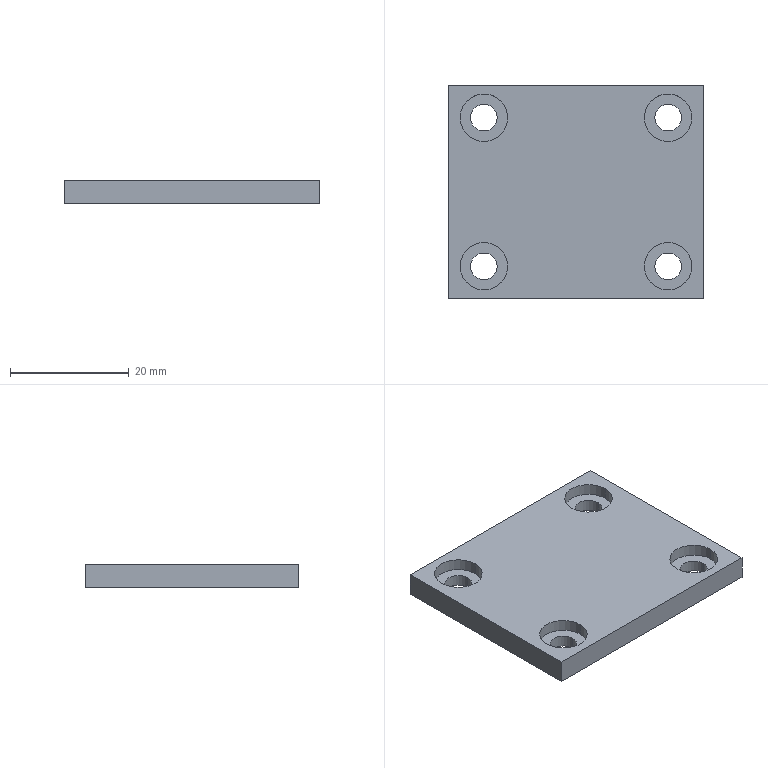Part | SolidWorks | features BaseBody 1 | 1 solid | 26 faces | box 43 x 36 x 4 mm | volume 5663 mm3 | cylinder 16 | plane 10 | commonest cylinder face diameters 4.5 x8 8 x8
STEP:
#1=CARTESIAN_POINT('',(-13.25,-12.5,0.));
#2=VERTEX_POINT('',#1);
#3=CARTESIAN_POINT('',(-17.75,-12.5,0.));
#4=VERTEX_POINT('',#3);
#5=CARTESIAN_POINT('',(-15.5,-12.5,0.));
#6=DIRECTION('',(0.,0.,-1.));
#7=DIRECTION('',(1.,0.,0.));
#8=AXIS2_PLACEMENT_3D('',#5,#6,#7);
#9=CIRCLE('',#8,2.25);
#10=EDGE_CURVE('',#2,#4,#9,.T.);
#11=ORIENTED_EDGE('',*,*,#10,.T.);
#12=CARTESIAN_POINT('',(-17.75,-12.5,2.));
#13=VERTEX_POINT('',#12);
#14=CARTESIAN_POINT('',(-17.75,-12.5,4.));
#15=DIRECTION('',(0.,0.,1.));
#16=VECTOR('',#15,1000.);
#17=LINE('',#14,#16);
#18=EDGE_CURVE('',#4,#13,#17,.T.);
#19=ORIENTED_EDGE('',*,*,#18,.T.);
#20=CARTESIAN_POINT('',(-13.25,-12.5,2.));
#21=VERTEX_POINT('',#20);
#22=CARTESIAN_POINT('',(-15.5,-12.5,2.));
#23=DIRECTION('',(0.,0.,-1.));
#24=DIRECTION('',(1.,0.,0.));
#25=AXIS2_PLACEMENT_3D('',#22,#23,#24);
#26=CIRCLE('',#25,2.25);
#27=EDGE_CURVE('',#21,#13,#26,.T.);
#28=ORIENTED_EDGE('',*,*,#27,.F.);
#29=CARTESIAN_POINT('',(-13.25,-12.5,4.));
#30=DIRECTION('',(0.,0.,1.));
#31=VECTOR('',#30,1000.);
#32=LINE('',#29,#31);
#33=EDGE_CURVE('',#2,#21,#32,.T.);
#34=ORIENTED_EDGE('',*,*,#33,.F.);
#35=EDGE_LOOP('',(#11,#19,#28,#34));
#36=FACE_OUTER_BOUND('',#35,.T.);
#37=CARTESIAN_POINT('',(-15.5,-12.5,4.));
#38=DIRECTION('',(0.,0.,1.));
#39=DIRECTION('',(1.,0.,0.));
#40=AXIS2_PLACEMENT_3D('',#37,#38,#39);
#41=CYLINDRICAL_SURFACE('',#40,2.25);
#42=ADVANCED_FACE('',(#36),#41,.F.);
#43=CARTESIAN_POINT('',(17.75,-12.5,0.));
#44=VERTEX_POINT('',#43);
#45=CARTESIAN_POINT('',(13.25,-12.5,0.));
#46=VERTEX_POINT('',#45);
#47=CARTESIAN_POINT('',(15.5,-12.5,0.));
#48=DIRECTION('',(0.,0.,-1.));
#49=DIRECTION('',(1.,0.,0.));
#50=AXIS2_PLACEMENT_3D('',#47,#48,#49);
#51=CIRCLE('',#50,2.25);
#52=EDGE_CURVE('',#44,#46,#51,.T.);
#53=ORIENTED_EDGE('',*,*,#52,.T.);
#54=CARTESIAN_POINT('',(13.25,-12.5,2.));
#55=VERTEX_POINT('',#54);
#56=CARTESIAN_POINT('',(13.25,-12.5,4.));
#57=DIRECTION('',(0.,0.,1.));
#58=VECTOR('',#57,1000.);
#59=LINE('',#56,#58);
#60=EDGE_CURVE('',#46,#55,#59,.T.);
#61=ORIENTED_EDGE('',*,*,#60,.T.);
#62=CARTESIAN_POINT('',(17.75,-12.5,2.));
#63=VERTEX_POINT('',#62);
#64=CARTESIAN_POINT('',(15.5,-12.5,2.));
#65=DIRECTION('',(0.,0.,-1.));
#66=DIRECTION('',(1.,0.,0.));
#67=AXIS2_PLACEMENT_3D('',#64,#65,#66);
#68=CIRCLE('',#67,2.25);
#69=EDGE_CURVE('',#63,#55,#68,.T.);
#70=ORIENTED_EDGE('',*,*,#69,.F.);
#71=CARTESIAN_POINT('',(17.75,-12.5,4.));
#72=DIRECTION('',(0.,0.,1.));
#73=VECTOR('',#72,1000.);
#74=LINE('',#71,#73);
#75=EDGE_CURVE('',#44,#63,#74,.T.);
#76=ORIENTED_EDGE('',*,*,#75,.F.);
#77=EDGE_LOOP('',(#53,#61,#70,#76));
#78=FACE_OUTER_BOUND('',#77,.T.);
#79=CARTESIAN_POINT('',(15.5,-12.5,4.));
#80=DIRECTION('',(0.,0.,1.));
#81=DIRECTION('',(1.,0.,0.));
#82=AXIS2_PLACEMENT_3D('',#79,#80,#81);
#83=CYLINDRICAL_SURFACE('',#82,2.25);
#84=ADVANCED_FACE('',(#78),#83,.F.);
#85=CARTESIAN_POINT('',(17.75,12.5,0.));
#86=VERTEX_POINT('',#85);
#87=CARTESIAN_POINT('',(13.25,12.5,0.));
#88=VERTEX_POINT('',#87);
#89=CARTESIAN_POINT('',(15.5,12.5,0.));
#90=DIRECTION('',(0.,0.,-1.));
#91=DIRECTION('',(1.,0.,0.));
#92=AXIS2_PLACEMENT_3D('',#89,#90,#91);
#93=CIRCLE('',#92,2.25);
#94=EDGE_CURVE('',#86,#88,#93,.T.);
#95=ORIENTED_EDGE('',*,*,#94,.T.);
#96=CARTESIAN_POINT('',(13.25,12.5,2.));
#97=VERTEX_POINT('',#96);
#98=CARTESIAN_POINT('',(13.25,12.5,4.));
#99=DIRECTION('',(0.,0.,1.));
#100=VECTOR('',#99,1000.);
#101=LINE('',#98,#100);
#102=EDGE_CURVE('',#88,#97,#101,.T.);
#103=ORIENTED_EDGE('',*,*,#102,.T.);
#104=CARTESIAN_POINT('',(17.75,12.5,2.));
#105=VERTEX_POINT('',#104);
#106=CARTESIAN_POINT('',(15.5,12.5,2.));
#107=DIRECTION('',(0.,0.,-1.));
#108=DIRECTION('',(1.,0.,0.));
#109=AXIS2_PLACEMENT_3D('',#106,#107,#108);
#110=CIRCLE('',#109,2.25);
#111=EDGE_CURVE('',#105,#97,#110,.T.);
#112=ORIENTED_EDGE('',*,*,#111,.F.);
#113=CARTESIAN_POINT('',(17.75,12.5,4.));
#114=DIRECTION('',(0.,0.,1.));
#115=VECTOR('',#114,1000.);
#116=LINE('',#113,#115);
#117=EDGE_CURVE('',#86,#105,#116,.T.);
#118=ORIENTED_EDGE('',*,*,#117,.F.);
#119=EDGE_LOOP('',(#95,#103,#112,#118));
#120=FACE_OUTER_BOUND('',#119,.T.);
#121=CARTESIAN_POINT('',(15.5,12.5,4.));
#122=DIRECTION('',(0.,0.,1.));
#123=DIRECTION('',(1.,0.,0.));
#124=AXIS2_PLACEMENT_3D('',#121,#122,#123);
#125=CYLINDRICAL_SURFACE('',#124,2.25);
#126=ADVANCED_FACE('',(#120),#125,.F.);
#127=CARTESIAN_POINT('',(-13.25,12.5,0.));
#128=VERTEX_POINT('',#127);
#129=CARTESIAN_POINT('',(-17.75,12.5,0.));
#130=VERTEX_POINT('',#129);
#131=CARTESIAN_POINT('',(-15.5,12.5,0.));
#132=DIRECTION('',(0.,0.,-1.));
#133=DIRECTION('',(1.,0.,0.));
#134=AXIS2_PLACEMENT_3D('',#131,#132,#133);
#135=CIRCLE('',#134,2.25);
#136=EDGE_CURVE('',#128,#130,#135,.T.);
#137=ORIENTED_EDGE('',*,*,#136,.T.);
#138=CARTESIAN_POINT('',(-17.75,12.5,2.));
#139=VERTEX_POINT('',#138);
#140=CARTESIAN_POINT('',(-17.75,12.5,4.));
#141=DIRECTION('',(0.,0.,1.));
#142=VECTOR('',#141,1000.);
#143=LINE('',#140,#142);
#144=EDGE_CURVE('',#130,#139,#143,.T.);
#145=ORIENTED_EDGE('',*,*,#144,.T.);
#146=CARTESIAN_POINT('',(-13.25,12.5,2.));
#147=VERTEX_POINT('',#146);
#148=CARTESIAN_POINT('',(-15.5,12.5,2.));
#149=DIRECTION('',(0.,0.,-1.));
#150=DIRECTION('',(1.,0.,0.));
#151=AXIS2_PLACEMENT_3D('',#148,#149,#150);
#152=CIRCLE('',#151,2.25);
#153=EDGE_CURVE('',#147,#139,#152,.T.);
#154=ORIENTED_EDGE('',*,*,#153,.F.);
#155=CARTESIAN_POINT('',(-13.25,12.5,4.));
#156=DIRECTION('',(0.,0.,1.));
#157=VECTOR('',#156,1000.);
#158=LINE('',#155,#157);
#159=EDGE_CURVE('',#128,#147,#158,.T.);
#160=ORIENTED_EDGE('',*,*,#159,.F.);
#161=EDGE_LOOP('',(#137,#145,#154,#160));
#162=FACE_OUTER_BOUND('',#161,.T.);
#163=CARTESIAN_POINT('',(-15.5,12.5,4.));
#164=DIRECTION('',(0.,0.,1.));
#165=DIRECTION('',(1.,0.,0.));
#166=AXIS2_PLACEMENT_3D('',#163,#164,#165);
#167=CYLINDRICAL_SURFACE('',#166,2.25);
#168=ADVANCED_FACE('',(#162),#167,.F.);
#169=CARTESIAN_POINT('',(-11.5,-12.5,2.));
#170=VERTEX_POINT('',#169);
#171=CARTESIAN_POINT('',(-19.5,-12.5,2.));
#172=VERTEX_POINT('',#171);
#173=CARTESIAN_POINT('',(-15.5,-12.5,2.));
#174=DIRECTION('',(0.,0.,-1.));
#175=DIRECTION('',(1.,0.,0.));
#176=AXIS2_PLACEMENT_3D('',#173,#174,#175);
#177=CIRCLE('',#176,4.);
#178=EDGE_CURVE('',#170,#172,#177,.T.);
#179=ORIENTED_EDGE('',*,*,#178,.T.);
#180=CARTESIAN_POINT('',(-19.5,-12.5,4.));
#181=VERTEX_POINT('',#180);
#182=CARTESIAN_POINT('',(-19.5,-12.5,4.));
#183=DIRECTION('',(0.,0.,1.));
#184=VECTOR('',#183,1000.);
#185=LINE('',#182,#184);
#186=EDGE_CURVE('',#172,#181,#185,.T.);
#187=ORIENTED_EDGE('',*,*,#186,.T.);
#188=CARTESIAN_POINT('',(-11.5,-12.5,4.));
#189=VERTEX_POINT('',#188);
#190=CARTESIAN_POINT('',(-15.5,-12.5,4.));
#191=DIRECTION('',(0.,0.,-1.));
#192=DIRECTION('',(1.,0.,0.));
#193=AXIS2_PLACEMENT_3D('',#190,#191,#192);
#194=CIRCLE('',#193,4.);
#195=EDGE_CURVE('',#189,#181,#194,.T.);
#196=ORIENTED_EDGE('',*,*,#195,.F.);
#197=CARTESIAN_POINT('',(-11.5,-12.5,4.));
#198=DIRECTION('',(0.,0.,1.));
#199=VECTOR('',#198,1000.);
#200=LINE('',#197,#199);
#201=EDGE_CURVE('',#170,#189,#200,.T.);
#202=ORIENTED_EDGE('',*,*,#201,.F.);
#203=EDGE_LOOP('',(#179,#187,#196,#202));
#204=FACE_OUTER_BOUND('',#203,.T.);
#205=CARTESIAN_POINT('',(-15.5,-12.5,4.));
#206=DIRECTION('',(0.,0.,1.));
#207=DIRECTION('',(1.,0.,0.));
#208=AXIS2_PLACEMENT_3D('',#205,#206,#207);
#209=CYLINDRICAL_SURFACE('',#208,4.);
#210=ADVANCED_FACE('',(#204),#209,.F.);
#211=CARTESIAN_POINT('',(19.5,-12.5,2.));
#212=VERTEX_POINT('',#211);
#213=CARTESIAN_POINT('',(11.5,-12.5,2.));
#214=VERTEX_POINT('',#213);
#215=CARTESIAN_POINT('',(15.5,-12.5,2.));
#216=DIRECTION('',(0.,0.,-1.));
#217=DIRECTION('',(1.,0.,0.));
#218=AXIS2_PLACEMENT_3D('',#215,#216,#217);
#219=CIRCLE('',#218,4.);
#220=EDGE_CURVE('',#212,#214,#219,.T.);
#221=ORIENTED_EDGE('',*,*,#220,.T.);
#222=CARTESIAN_POINT('',(11.5,-12.5,4.));
#223=VERTEX_POINT('',#222);
#224=CARTESIAN_POINT('',(11.5,-12.5,4.));
#225=DIRECTION('',(0.,0.,1.));
#226=VECTOR('',#225,1000.);
#227=LINE('',#224,#226);
#228=EDGE_CURVE('',#214,#223,#227,.T.);
#229=ORIENTED_EDGE('',*,*,#228,.T.);
#230=CARTESIAN_POINT('',(19.5,-12.5,4.));
#231=VERTEX_POINT('',#230);
#232=CARTESIAN_POINT('',(15.5,-12.5,4.));
#233=DIRECTION('',(0.,0.,-1.));
#234=DIRECTION('',(1.,0.,0.));
#235=AXIS2_PLACEMENT_3D('',#232,#233,#234);
#236=CIRCLE('',#235,4.);
#237=EDGE_CURVE('',#231,#223,#236,.T.);
#238=ORIENTED_EDGE('',*,*,#237,.F.);
#239=CARTESIAN_POINT('',(19.5,-12.5,4.));
#240=DIRECTION('',(0.,0.,1.));
#241=VECTOR('',#240,1000.);
#242=LINE('',#239,#241);
#243=EDGE_CURVE('',#212,#231,#242,.T.);
#244=ORIENTED_EDGE('',*,*,#243,.F.);
#245=EDGE_LOOP('',(#221,#229,#238,#244));
#246=FACE_OUTER_BOUND('',#245,.T.);
#247=CARTESIAN_POINT('',(15.5,-12.5,4.));
#248=DIRECTION('',(0.,0.,1.));
#249=DIRECTION('',(1.,0.,0.));
#250=AXIS2_PLACEMENT_3D('',#247,#248,#249);
#251=CYLINDRICAL_SURFACE('',#250,4.);
#252=ADVANCED_FACE('',(#246),#251,.F.);
#253=CARTESIAN_POINT('',(19.5,12.5,2.));
#254=VERTEX_POINT('',#253);
#255=CARTESIAN_POINT('',(11.5,12.5,2.));
#256=VERTEX_POINT('',#255);
#257=CARTESIAN_POINT('',(15.5,12.5,2.));
#258=DIRECTION('',(0.,0.,-1.));
#259=DIRECTION('',(1.,0.,0.));
#260=AXIS2_PLACEMENT_3D('',#257,#258,#259);
#261=CIRCLE('',#260,4.);
#262=EDGE_CURVE('',#254,#256,#261,.T.);
#263=ORIENTED_EDGE('',*,*,#262,.T.);
#264=CARTESIAN_POINT('',(11.5,12.5,4.));
#265=VERTEX_POINT('',#264);
#266=CARTESIAN_POINT('',(11.5,12.5,4.));
#267=DIRECTION('',(0.,0.,1.));
#268=VECTOR('',#267,1000.);
#269=LINE('',#266,#268);
#270=EDGE_CURVE('',#256,#265,#269,.T.);
#271=ORIENTED_EDGE('',*,*,#270,.T.);
#272=CARTESIAN_POINT('',(19.5,12.5,4.));
#273=VERTEX_POINT('',#272);
#274=CARTESIAN_POINT('',(15.5,12.5,4.));
#275=DIRECTION('',(0.,0.,-1.));
#276=DIRECTION('',(1.,0.,0.));
#277=AXIS2_PLACEMENT_3D('',#274,#275,#276);
#278=CIRCLE('',#277,4.);
#279=EDGE_CURVE('',#273,#265,#278,.T.);
#280=ORIENTED_EDGE('',*,*,#279,.F.);
#281=CARTESIAN_POINT('',(19.5,12.5,4.));
#282=DIRECTION('',(0.,0.,1.));
#283=VECTOR('',#282,1000.);
#284=LINE('',#281,#283);
#285=EDGE_CURVE('',#254,#273,#284,.T.);
#286=ORIENTED_EDGE('',*,*,#285,.F.);
#287=EDGE_LOOP('',(#263,#271,#280,#286));
#288=FACE_OUTER_BOUND('',#287,.T.);
#289=CARTESIAN_POINT('',(15.5,12.5,4.));
#290=DIRECTION('',(0.,0.,1.));
#291=DIRECTION('',(1.,0.,0.));
#292=AXIS2_PLACEMENT_3D('',#289,#290,#291);
#293=CYLINDRICAL_SURFACE('',#292,4.);
#294=ADVANCED_FACE('',(#288),#293,.F.);
#295=CARTESIAN_POINT('',(-11.5,12.5,2.));
#296=VERTEX_POINT('',#295);
#297=CARTESIAN_POINT('',(-19.5,12.5,2.));
#298=VERTEX_POINT('',#297);
#299=CARTESIAN_POINT('',(-15.5,12.5,2.));
#300=DIRECTION('',(0.,0.,-1.));
#301=DIRECTION('',(1.,0.,0.));
#302=AXIS2_PLACEMENT_3D('',#299,#300,#301);
#303=CIRCLE('',#302,4.);
#304=EDGE_CURVE('',#296,#298,#303,.T.);
#305=ORIENTED_EDGE('',*,*,#304,.T.);
#306=CARTESIAN_POINT('',(-19.5,12.5,4.));
#307=VERTEX_POINT('',#306);
#308=CARTESIAN_POINT('',(-19.5,12.5,4.));
#309=DIRECTION('',(0.,0.,1.));
#310=VECTOR('',#309,1000.);
#311=LINE('',#308,#310);
#312=EDGE_CURVE('',#298,#307,#311,.T.);
#313=ORIENTED_EDGE('',*,*,#312,.T.);
#314=CARTESIAN_POINT('',(-11.5,12.5,4.));
#315=VERTEX_POINT('',#314);
#316=CARTESIAN_POINT('',(-15.5,12.5,4.));
#317=DIRECTION('',(0.,0.,-1.));
#318=DIRECTION('',(1.,0.,0.));
#319=AXIS2_PLACEMENT_3D('',#316,#317,#318);
#320=CIRCLE('',#319,4.);
#321=EDGE_CURVE('',#315,#307,#320,.T.);
#322=ORIENTED_EDGE('',*,*,#321,.F.);
#323=CARTESIAN_POINT('',(-11.5,12.5,4.));
#324=DIRECTION('',(0.,0.,1.));
#325=VECTOR('',#324,1000.);
#326=LINE('',#323,#325);
#327=EDGE_CURVE('',#296,#315,#326,.T.);
#328=ORIENTED_EDGE('',*,*,#327,.F.);
#329=EDGE_LOOP('',(#305,#313,#322,#328));
#330=FACE_OUTER_BOUND('',#329,.T.);
#331=CARTESIAN_POINT('',(-15.5,12.5,4.));
#332=DIRECTION('',(0.,0.,1.));
#333=DIRECTION('',(1.,0.,0.));
#334=AXIS2_PLACEMENT_3D('',#331,#332,#333);
#335=CYLINDRICAL_SURFACE('',#334,4.);
#336=ADVANCED_FACE('',(#330),#335,.F.);
#337=CARTESIAN_POINT('',(-21.5,-18.,0.));
#338=VERTEX_POINT('',#337);
#339=CARTESIAN_POINT('',(21.5,-18.,0.));
#340=VERTEX_POINT('',#339);
#341=CARTESIAN_POINT('',(0.,-18.,0.));
#342=DIRECTION('',(1.,0.,0.));
#343=VECTOR('',#342,1000.);
#344=LINE('',#341,#343);
#345=EDGE_CURVE('',#338,#340,#344,.T.);
#346=ORIENTED_EDGE('',*,*,#345,.F.);
#347=CARTESIAN_POINT('',(-21.5,18.,0.));
#348=VERTEX_POINT('',#347);
#349=CARTESIAN_POINT('',(-21.5,0.,0.));
#350=DIRECTION('',(0.,-1.,0.));
#351=VECTOR('',#350,1000.);
#352=LINE('',#349,#351);
#353=EDGE_CURVE('',#348,#338,#352,.T.);
#354=ORIENTED_EDGE('',*,*,#353,.F.);
#355=CARTESIAN_POINT('',(21.5,18.,0.));
#356=VERTEX_POINT('',#355);
#357=CARTESIAN_POINT('',(0.,18.,0.));
#358=DIRECTION('',(-1.,0.,0.));
#359=VECTOR('',#358,1000.);
#360=LINE('',#357,#359);
#361=EDGE_CURVE('',#356,#348,#360,.T.);
#362=ORIENTED_EDGE('',*,*,#361,.F.);
#363=CARTESIAN_POINT('',(21.5,0.,0.));
#364=DIRECTION('',(0.,1.,0.));
#365=VECTOR('',#364,1000.);
#366=LINE('',#363,#365);
#367=EDGE_CURVE('',#340,#356,#366,.T.);
#368=ORIENTED_EDGE('',*,*,#367,.F.);
#369=EDGE_LOOP('',(#346,#354,#362,#368));
#370=FACE_OUTER_BOUND('',#369,.T.);
#371=ORIENTED_EDGE('',*,*,#10,.F.);
#372=CARTESIAN_POINT('',(-15.5,-12.5,0.));
#373=DIRECTION('',(0.,0.,-1.));
#374=DIRECTION('',(1.,0.,0.));
#375=AXIS2_PLACEMENT_3D('',#372,#373,#374);
#376=CIRCLE('',#375,2.25);
#377=EDGE_CURVE('',#4,#2,#376,.T.);
#378=ORIENTED_EDGE('',*,*,#377,.F.);
#379=EDGE_LOOP('',(#371,#378));
#380=FACE_BOUND('',#379,.T.);
#381=ORIENTED_EDGE('',*,*,#52,.F.);
#382=CARTESIAN_POINT('',(15.5,-12.5,0.));
#383=DIRECTION('',(0.,0.,-1.));
#384=DIRECTION('',(1.,0.,0.));
#385=AXIS2_PLACEMENT_3D('',#382,#383,#384);
#386=CIRCLE('',#385,2.25);
#387=EDGE_CURVE('',#46,#44,#386,.T.);
#388=ORIENTED_EDGE('',*,*,#387,.F.);
#389=EDGE_LOOP('',(#381,#388));
#390=FACE_BOUND('',#389,.T.);
#391=ORIENTED_EDGE('',*,*,#94,.F.);
#392=CARTESIAN_POINT('',(15.5,12.5,0.));
#393=DIRECTION('',(0.,0.,-1.));
#394=DIRECTION('',(1.,0.,0.));
#395=AXIS2_PLACEMENT_3D('',#392,#393,#394);
#396=CIRCLE('',#395,2.25);
#397=EDGE_CURVE('',#88,#86,#396,.T.);
#398=ORIENTED_EDGE('',*,*,#397,.F.);
#399=EDGE_LOOP('',(#391,#398));
#400=FACE_BOUND('',#399,.T.);
#401=ORIENTED_EDGE('',*,*,#136,.F.);
#402=CARTESIAN_POINT('',(-15.5,12.5,0.));
#403=DIRECTION('',(0.,0.,-1.));
#404=DIRECTION('',(1.,0.,0.));
#405=AXIS2_PLACEMENT_3D('',#402,#403,#404);
#406=CIRCLE('',#405,2.25);
#407=EDGE_CURVE('',#130,#128,#406,.T.);
#408=ORIENTED_EDGE('',*,*,#407,.F.);
#409=EDGE_LOOP('',(#401,#408));
#410=FACE_BOUND('',#409,.T.);
#411=CARTESIAN_POINT('',(0.,0.,0.));
#412=DIRECTION('',(0.,0.,1.));
#413=DIRECTION('',(1.,0.,0.));
#414=AXIS2_PLACEMENT_3D('',#411,#412,#413);
#415=PLANE('',#414);
#416=ADVANCED_FACE('',(#370,#380,#390,#400,#410),#415,.F.);
#417=CARTESIAN_POINT('',(21.5,18.,4.));
#418=VERTEX_POINT('',#417);
#419=CARTESIAN_POINT('',(21.5,18.,4.));
#420=DIRECTION('',(0.,0.,-1.));
#421=VECTOR('',#420,1000.);
#422=LINE('',#419,#421);
#423=EDGE_CURVE('',#418,#356,#422,.T.);
#424=ORIENTED_EDGE('',*,*,#423,.F.);
#425=CARTESIAN_POINT('',(21.5,-18.,4.));
#426=VERTEX_POINT('',#425);
#427=CARTESIAN_POINT('',(21.5,18.,4.));
#428=DIRECTION('',(0.,1.,0.));
#429=VECTOR('',#428,1000.);
#430=LINE('',#427,#429);
#431=EDGE_CURVE('',#426,#418,#430,.T.);
#432=ORIENTED_EDGE('',*,*,#431,.F.);
#433=CARTESIAN_POINT('',(21.5,-18.,4.));
#434=DIRECTION('',(0.,0.,1.));
#435=VECTOR('',#434,1000.);
#436=LINE('',#433,#435);
#437=EDGE_CURVE('',#340,#426,#436,.T.);
#438=ORIENTED_EDGE('',*,*,#437,.F.);
#439=ORIENTED_EDGE('',*,*,#367,.T.);
#440=EDGE_LOOP('',(#424,#432,#438,#439));
#441=FACE_OUTER_BOUND('',#440,.T.);
#442=CARTESIAN_POINT('',(21.5,18.,4.));
#443=DIRECTION('',(-1.,0.,0.));
#444=DIRECTION('',(0.,-1.,0.));
#445=AXIS2_PLACEMENT_3D('',#442,#443,#444);
#446=PLANE('',#445);
#447=ADVANCED_FACE('',(#441),#446,.F.);
#448=ORIENTED_EDGE('',*,*,#437,.T.);
#449=CARTESIAN_POINT('',(-21.5,-18.,4.));
#450=VERTEX_POINT('',#449);
#451=CARTESIAN_POINT('',(-21.5,-18.,4.));
#452=DIRECTION('',(1.,0.,0.));
#453=VECTOR('',#452,1000.);
#454=LINE('',#451,#453);
#455=EDGE_CURVE('',#450,#426,#454,.T.);
#456=ORIENTED_EDGE('',*,*,#455,.F.);
#457=CARTESIAN_POINT('',(-21.5,-18.,4.));
#458=DIRECTION('',(0.,0.,1.));
#459=VECTOR('',#458,1000.);
#460=LINE('',#457,#459);
#461=EDGE_CURVE('',#338,#450,#460,.T.);
#462=ORIENTED_EDGE('',*,*,#461,.F.);
#463=ORIENTED_EDGE('',*,*,#345,.T.);
#464=EDGE_LOOP('',(#448,#456,#462,#463));
#465=FACE_OUTER_BOUND('',#464,.T.);
#466=CARTESIAN_POINT('',(-21.5,-18.,4.));
#467=DIRECTION('',(0.,1.,0.));
#468=DIRECTION('',(0.,0.,1.));
#469=AXIS2_PLACEMENT_3D('',#466,#467,#468);
#470=PLANE('',#469);
#471=ADVANCED_FACE('',(#465),#470,.F.);
#472=ORIENTED_EDGE('',*,*,#461,.T.);
#473=CARTESIAN_POINT('',(-21.5,18.,4.));
#474=VERTEX_POINT('',#473);
#475=CARTESIAN_POINT('',(-21.5,18.,4.));
#476=DIRECTION('',(0.,-1.,0.));
#477=VECTOR('',#476,1000.);
#478=LINE('',#475,#477);
#479=EDGE_CURVE('',#474,#450,#478,.T.);
#480=ORIENTED_EDGE('',*,*,#479,.F.);
#481=CARTESIAN_POINT('',(-21.5,18.,4.));
#482=DIRECTION('',(0.,0.,1.));
#483=VECTOR('',#482,1000.);
#484=LINE('',#481,#483);
#485=EDGE_CURVE('',#348,#474,#484,.T.);
#486=ORIENTED_EDGE('',*,*,#485,.F.);
#487=ORIENTED_EDGE('',*,*,#353,.T.);
#488=EDGE_LOOP('',(#472,#480,#486,#487));
#489=FACE_OUTER_BOUND('',#488,.T.);
#490=CARTESIAN_POINT('',(-21.5,18.,4.));
#491=DIRECTION('',(1.,0.,0.));
#492=DIRECTION('',(0.,0.,-1.));
#493=AXIS2_PLACEMENT_3D('',#490,#491,#492);
#494=PLANE('',#493);
#495=ADVANCED_FACE('',(#489),#494,.F.);
#496=ORIENTED_EDGE('',*,*,#485,.T.);
#497=CARTESIAN_POINT('',(-21.5,18.,4.));
#498=DIRECTION('',(-1.,0.,0.));
#499=VECTOR('',#498,1000.);
#500=LINE('',#497,#499);
#501=EDGE_CURVE('',#418,#474,#500,.T.);
#502=ORIENTED_EDGE('',*,*,#501,.F.);
#503=ORIENTED_EDGE('',*,*,#423,.T.);
#504=ORIENTED_EDGE('',*,*,#361,.T.);
#505=EDGE_LOOP('',(#496,#502,#503,#504));
#506=FACE_OUTER_BOUND('',#505,.T.);
#507=CARTESIAN_POINT('',(-21.5,18.,4.));
#508=DIRECTION('',(0.,-1.,0.));
#509=DIRECTION('',(0.,0.,-1.));
#510=AXIS2_PLACEMENT_3D('',#507,#508,#509);
#511=PLANE('',#510);
#512=ADVANCED_FACE('',(#506),#511,.F.);
#513=ORIENTED_EDGE('',*,*,#18,.F.);
#514=ORIENTED_EDGE('',*,*,#377,.T.);
#515=ORIENTED_EDGE('',*,*,#33,.T.);
#516=CARTESIAN_POINT('',(-15.5,-12.5,2.));
#517=DIRECTION('',(0.,0.,-1.));
#518=DIRECTION('',(1.,0.,0.));
#519=AXIS2_PLACEMENT_3D('',#516,#517,#518);
#520=CIRCLE('',#519,2.25);
#521=EDGE_CURVE('',#13,#21,#520,.T.);
#522=ORIENTED_EDGE('',*,*,#521,.F.);
#523=EDGE_LOOP('',(#513,#514,#515,#522));
#524=FACE_OUTER_BOUND('',#523,.T.);
#525=CARTESIAN_POINT('',(-15.5,-12.5,4.));
#526=DIRECTION('',(0.,0.,1.));
#527=DIRECTION('',(1.,0.,0.));
#528=AXIS2_PLACEMENT_3D('',#525,#526,#527);
#529=CYLINDRICAL_SURFACE('',#528,2.25);
#530=ADVANCED_FACE('',(#524),#529,.F.);
#531=ORIENTED_EDGE('',*,*,#60,.F.);
#532=ORIENTED_EDGE('',*,*,#387,.T.);
#533=ORIENTED_EDGE('',*,*,#75,.T.);
#534=CARTESIAN_POINT('',(15.5,-12.5,2.));
#535=DIRECTION('',(0.,0.,-1.));
#536=DIRECTION('',(1.,0.,0.));
#537=AXIS2_PLACEMENT_3D('',#534,#535,#536);
#538=CIRCLE('',#537,2.25);
#539=EDGE_CURVE('',#55,#63,#538,.T.);
#540=ORIENTED_EDGE('',*,*,#539,.F.);
#541=EDGE_LOOP('',(#531,#532,#533,#540));
#542=FACE_OUTER_BOUND('',#541,.T.);
#543=CARTESIAN_POINT('',(15.5,-12.5,4.));
#544=DIRECTION('',(0.,0.,1.));
#545=DIRECTION('',(1.,0.,0.));
#546=AXIS2_PLACEMENT_3D('',#543,#544,#545);
#547=CYLINDRICAL_SURFACE('',#546,2.25);
#548=ADVANCED_FACE('',(#542),#547,.F.);
#549=ORIENTED_EDGE('',*,*,#102,.F.);
#550=ORIENTED_EDGE('',*,*,#397,.T.);
#551=ORIENTED_EDGE('',*,*,#117,.T.);
#552=CARTESIAN_POINT('',(15.5,12.5,2.));
#553=DIRECTION('',(0.,0.,-1.));
#554=DIRECTION('',(1.,0.,0.));
#555=AXIS2_PLACEMENT_3D('',#552,#553,#554);
#556=CIRCLE('',#555,2.25);
#557=EDGE_CURVE('',#97,#105,#556,.T.);
#558=ORIENTED_EDGE('',*,*,#557,.F.);
#559=EDGE_LOOP('',(#549,#550,#551,#558));
#560=FACE_OUTER_BOUND('',#559,.T.);
#561=CARTESIAN_POINT('',(15.5,12.5,4.));
#562=DIRECTION('',(0.,0.,1.));
#563=DIRECTION('',(1.,0.,0.));
#564=AXIS2_PLACEMENT_3D('',#561,#562,#563);
#565=CYLINDRICAL_SURFACE('',#564,2.25);
#566=ADVANCED_FACE('',(#560),#565,.F.);
#567=ORIENTED_EDGE('',*,*,#144,.F.);
#568=ORIENTED_EDGE('',*,*,#407,.T.);
#569=ORIENTED_EDGE('',*,*,#159,.T.);
#570=CARTESIAN_POINT('',(-15.5,12.5,2.));
#571=DIRECTION('',(0.,0.,-1.));
#572=DIRECTION('',(1.,0.,0.));
#573=AXIS2_PLACEMENT_3D('',#570,#571,#572);
#574=CIRCLE('',#573,2.25);
#575=EDGE_CURVE('',#139,#147,#574,.T.);
#576=ORIENTED_EDGE('',*,*,#575,.F.);
#577=EDGE_LOOP('',(#567,#568,#569,#576));
#578=FACE_OUTER_BOUND('',#577,.T.);
#579=CARTESIAN_POINT('',(-15.5,12.5,4.));
#580=DIRECTION('',(0.,0.,1.));
#581=DIRECTION('',(1.,0.,0.));
#582=AXIS2_PLACEMENT_3D('',#579,#580,#581);
#583=CYLINDRICAL_SURFACE('',#582,2.25);
#584=ADVANCED_FACE('',(#578),#583,.F.);
#585=ORIENTED_EDGE('',*,*,#479,.T.);
#586=ORIENTED_EDGE('',*,*,#455,.T.);
#587=ORIENTED_EDGE('',*,*,#431,.T.);
#588=ORIENTED_EDGE('',*,*,#501,.T.);
#589=EDGE_LOOP('',(#585,#586,#587,#588));
#590=FACE_OUTER_BOUND('',#589,.T.);
#591=ORIENTED_EDGE('',*,*,#195,.T.);
#592=CARTESIAN_POINT('',(-15.5,-12.5,4.));
#593=DIRECTION('',(0.,0.,-1.));
#594=DIRECTION('',(1.,0.,0.));
#595=AXIS2_PLACEMENT_3D('',#592,#593,#594);
#596=CIRCLE('',#595,4.);
#597=EDGE_CURVE('',#181,#189,#596,.T.);
#598=ORIENTED_EDGE('',*,*,#597,.T.);
#599=EDGE_LOOP('',(#591,#598));
#600=FACE_BOUND('',#599,.T.);
#601=ORIENTED_EDGE('',*,*,#237,.T.);
#602=CARTESIAN_POINT('',(15.5,-12.5,4.));
#603=DIRECTION('',(0.,0.,-1.));
#604=DIRECTION('',(1.,0.,0.));
#605=AXIS2_PLACEMENT_3D('',#602,#603,#604);
#606=CIRCLE('',#605,4.);
#607=EDGE_CURVE('',#223,#231,#606,.T.);
#608=ORIENTED_EDGE('',*,*,#607,.T.);
#609=EDGE_LOOP('',(#601,#608));
#610=FACE_BOUND('',#609,.T.);
#611=ORIENTED_EDGE('',*,*,#279,.T.);
#612=CARTESIAN_POINT('',(15.5,12.5,4.));
#613=DIRECTION('',(0.,0.,-1.));
#614=DIRECTION('',(1.,0.,0.));
#615=AXIS2_PLACEMENT_3D('',#612,#613,#614);
#616=CIRCLE('',#615,4.);
#617=EDGE_CURVE('',#265,#273,#616,.T.);
#618=ORIENTED_EDGE('',*,*,#617,.T.);
#619=EDGE_LOOP('',(#611,#618));
#620=FACE_BOUND('',#619,.T.);
#621=ORIENTED_EDGE('',*,*,#321,.T.);
#622=CARTESIAN_POINT('',(-15.5,12.5,4.));
#623=DIRECTION('',(0.,0.,-1.));
#624=DIRECTION('',(1.,0.,0.));
#625=AXIS2_PLACEMENT_3D('',#622,#623,#624);
#626=CIRCLE('',#625,4.);
#627=EDGE_CURVE('',#307,#315,#626,.T.);
#628=ORIENTED_EDGE('',*,*,#627,.T.);
#629=EDGE_LOOP('',(#621,#628));
#630=FACE_BOUND('',#629,.T.);
#631=CARTESIAN_POINT('',(0.,0.,4.));
#632=DIRECTION('',(0.,0.,1.));
#633=DIRECTION('',(1.,0.,0.));
#634=AXIS2_PLACEMENT_3D('',#631,#632,#633);
#635=PLANE('',#634);
#636=ADVANCED_FACE('',(#590,#600,#610,#620,#630),#635,.T.);
#637=ORIENTED_EDGE('',*,*,#178,.F.);
#638=CARTESIAN_POINT('',(-15.5,-12.5,2.));
#639=DIRECTION('',(0.,0.,-1.));
#640=DIRECTION('',(1.,0.,0.));
#641=AXIS2_PLACEMENT_3D('',#638,#639,#640);
#642=CIRCLE('',#641,4.);
#643=EDGE_CURVE('',#172,#170,#642,.T.);
#644=ORIENTED_EDGE('',*,*,#643,.F.);
#645=EDGE_LOOP('',(#637,#644));
#646=FACE_OUTER_BOUND('',#645,.T.);
#647=ORIENTED_EDGE('',*,*,#27,.T.);
#648=ORIENTED_EDGE('',*,*,#521,.T.);
#649=EDGE_LOOP('',(#647,#648));
#650=FACE_BOUND('',#649,.T.);
#651=CARTESIAN_POINT('',(-13.25,-12.5,2.));
#652=DIRECTION('',(0.,0.,-1.));
#653=DIRECTION('',(-1.,0.,0.));
#654=AXIS2_PLACEMENT_3D('',#651,#652,#653);
#655=PLANE('',#654);
#656=ADVANCED_FACE('',(#646,#650),#655,.F.);
#657=ORIENTED_EDGE('',*,*,#220,.F.);
#658=CARTESIAN_POINT('',(15.5,-12.5,2.));
#659=DIRECTION('',(0.,0.,-1.));
#660=DIRECTION('',(1.,0.,0.));
#661=AXIS2_PLACEMENT_3D('',#658,#659,#660);
#662=CIRCLE('',#661,4.);
#663=EDGE_CURVE('',#214,#212,#662,.T.);
#664=ORIENTED_EDGE('',*,*,#663,.F.);
#665=EDGE_LOOP('',(#657,#664));
#666=FACE_OUTER_BOUND('',#665,.T.);
#667=ORIENTED_EDGE('',*,*,#69,.T.);
#668=ORIENTED_EDGE('',*,*,#539,.T.);
#669=EDGE_LOOP('',(#667,#668));
#670=FACE_BOUND('',#669,.T.);
#671=CARTESIAN_POINT('',(17.75,-12.5,2.));
#672=DIRECTION('',(0.,0.,-1.));
#673=DIRECTION('',(-1.,0.,0.));
#674=AXIS2_PLACEMENT_3D('',#671,#672,#673);
#675=PLANE('',#674);
#676=ADVANCED_FACE('',(#666,#670),#675,.F.);
#677=ORIENTED_EDGE('',*,*,#262,.F.);
#678=CARTESIAN_POINT('',(15.5,12.5,2.));
#679=DIRECTION('',(0.,0.,-1.));
#680=DIRECTION('',(1.,0.,0.));
#681=AXIS2_PLACEMENT_3D('',#678,#679,#680);
#682=CIRCLE('',#681,4.);
#683=EDGE_CURVE('',#256,#254,#682,.T.);
#684=ORIENTED_EDGE('',*,*,#683,.F.);
#685=EDGE_LOOP('',(#677,#684));
#686=FACE_OUTER_BOUND('',#685,.T.);
#687=ORIENTED_EDGE('',*,*,#111,.T.);
#688=ORIENTED_EDGE('',*,*,#557,.T.);
#689=EDGE_LOOP('',(#687,#688));
#690=FACE_BOUND('',#689,.T.);
#691=CARTESIAN_POINT('',(17.75,12.5,2.));
#692=DIRECTION('',(0.,0.,-1.));
#693=DIRECTION('',(-1.,0.,0.));
#694=AXIS2_PLACEMENT_3D('',#691,#692,#693);
#695=PLANE('',#694);
#696=ADVANCED_FACE('',(#686,#690),#695,.F.);
#697=ORIENTED_EDGE('',*,*,#304,.F.);
#698=CARTESIAN_POINT('',(-15.5,12.5,2.));
#699=DIRECTION('',(0.,0.,-1.));
#700=DIRECTION('',(1.,0.,0.));
#701=AXIS2_PLACEMENT_3D('',#698,#699,#700);
#702=CIRCLE('',#701,4.);
#703=EDGE_CURVE('',#298,#296,#702,.T.);
#704=ORIENTED_EDGE('',*,*,#703,.F.);
#705=EDGE_LOOP('',(#697,#704));
#706=FACE_OUTER_BOUND('',#705,.T.);
#707=ORIENTED_EDGE('',*,*,#153,.T.);
#708=ORIENTED_EDGE('',*,*,#575,.T.);
#709=EDGE_LOOP('',(#707,#708));
#710=FACE_BOUND('',#709,.T.);
#711=CARTESIAN_POINT('',(-13.25,12.5,2.));
#712=DIRECTION('',(0.,0.,-1.));
#713=DIRECTION('',(-1.,0.,0.));
#714=AXIS2_PLACEMENT_3D('',#711,#712,#713);
#715=PLANE('',#714);
#716=ADVANCED_FACE('',(#706,#710),#715,.F.);
#717=ORIENTED_EDGE('',*,*,#186,.F.);
#718=ORIENTED_EDGE('',*,*,#643,.T.);
#719=ORIENTED_EDGE('',*,*,#201,.T.);
#720=ORIENTED_EDGE('',*,*,#597,.F.);
#721=EDGE_LOOP('',(#717,#718,#719,#720));
#722=FACE_OUTER_BOUND('',#721,.T.);
#723=CARTESIAN_POINT('',(-15.5,-12.5,4.));
#724=DIRECTION('',(0.,0.,1.));
#725=DIRECTION('',(1.,0.,0.));
#726=AXIS2_PLACEMENT_3D('',#723,#724,#725);
#727=CYLINDRICAL_SURFACE('',#726,4.);
#728=ADVANCED_FACE('',(#722),#727,.F.);
#729=ORIENTED_EDGE('',*,*,#228,.F.);
#730=ORIENTED_EDGE('',*,*,#663,.T.);
#731=ORIENTED_EDGE('',*,*,#243,.T.);
#732=ORIENTED_EDGE('',*,*,#607,.F.);
#733=EDGE_LOOP('',(#729,#730,#731,#732));
#734=FACE_OUTER_BOUND('',#733,.T.);
#735=CARTESIAN_POINT('',(15.5,-12.5,4.));
#736=DIRECTION('',(0.,0.,1.));
#737=DIRECTION('',(1.,0.,0.));
#738=AXIS2_PLACEMENT_3D('',#735,#736,#737);
#739=CYLINDRICAL_SURFACE('',#738,4.);
#740=ADVANCED_FACE('',(#734),#739,.F.);
#741=ORIENTED_EDGE('',*,*,#270,.F.);
#742=ORIENTED_EDGE('',*,*,#683,.T.);
#743=ORIENTED_EDGE('',*,*,#285,.T.);
#744=ORIENTED_EDGE('',*,*,#617,.F.);
#745=EDGE_LOOP('',(#741,#742,#743,#744));
#746=FACE_OUTER_BOUND('',#745,.T.);
#747=CARTESIAN_POINT('',(15.5,12.5,4.));
#748=DIRECTION('',(0.,0.,1.));
#749=DIRECTION('',(1.,0.,0.));
#750=AXIS2_PLACEMENT_3D('',#747,#748,#749);
#751=CYLINDRICAL_SURFACE('',#750,4.);
#752=ADVANCED_FACE('',(#746),#751,.F.);
#753=ORIENTED_EDGE('',*,*,#312,.F.);
#754=ORIENTED_EDGE('',*,*,#703,.T.);
#755=ORIENTED_EDGE('',*,*,#327,.T.);
#756=ORIENTED_EDGE('',*,*,#627,.F.);
#757=EDGE_LOOP('',(#753,#754,#755,#756));
#758=FACE_OUTER_BOUND('',#757,.T.);
#759=CARTESIAN_POINT('',(-15.5,12.5,4.));
#760=DIRECTION('',(0.,0.,1.));
#761=DIRECTION('',(1.,0.,0.));
#762=AXIS2_PLACEMENT_3D('',#759,#760,#761);
#763=CYLINDRICAL_SURFACE('',#762,4.);
#764=ADVANCED_FACE('',(#758),#763,.F.);
#765=CLOSED_SHELL('',(#42,#84,#126,#168,#210,#252,#294,#336,#416,#447,#471,#495,#512,#530,#548,#566,#584,#636,#656,#676,#696,#716,#728,#740,#752,#764));
#766=MANIFOLD_SOLID_BREP('',#765);
#767=CARTESIAN_POINT('',(0.,0.,0.));
#768=DIRECTION('',(0.,0.,1.));
#769=DIRECTION('',(1.,0.,0.));
#770=AXIS2_PLACEMENT_3D('',#767,#768,#769);
#771=(LENGTH_UNIT()NAMED_UNIT(*)SI_UNIT(.MILLI.,.METRE.));
#772=UNCERTAINTY_MEASURE_WITH_UNIT(LENGTH_MEASURE(0.00001),#771,'','');
#773=(NAMED_UNIT(*)PLANE_ANGLE_UNIT()SI_UNIT($,.RADIAN.));
#774=(NAMED_UNIT(*)SI_UNIT($,.STERADIAN.)SOLID_ANGLE_UNIT());
#775=(GEOMETRIC_REPRESENTATION_CONTEXT(3)GLOBAL_UNCERTAINTY_ASSIGNED_CONTEXT((#772))GLOBAL_UNIT_ASSIGNED_CONTEXT((#771,#773,#774))REPRESENTATION_CONTEXT('',''));
#776=ADVANCED_BREP_SHAPE_REPRESENTATION('',(#766,#770),#775);